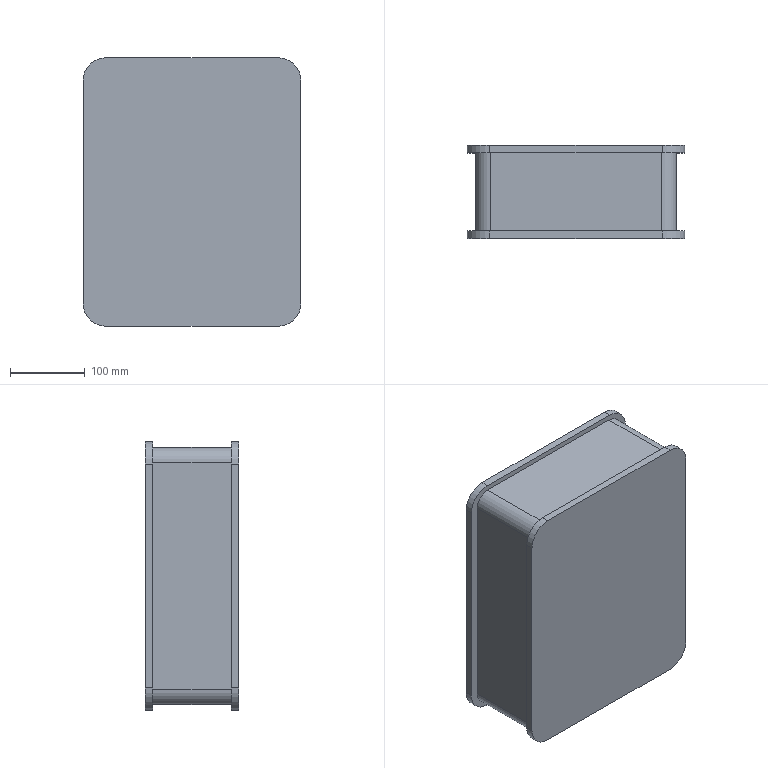Part | STEP file | CONTENEDOR TORNILLOS | 1 solid | 37 faces | box 292 x 125 x 360 mm | volume 3821373 mm3 | plane 21 | cylinder 16 | commonest cylinder face diameters 40 x8 60 x8
STEP:
#1=CARTESIAN_POINT('',(146.,125.,150.));
#2=VERTEX_POINT('',#1);
#3=CARTESIAN_POINT('',(146.,115.,150.));
#4=VERTEX_POINT('',#3);
#5=CARTESIAN_POINT('',(146.,125.,150.));
#6=DIRECTION('',(0.,-1.,0.));
#7=VECTOR('',#6,1000.);
#8=LINE('',#5,#7);
#9=EDGE_CURVE('',#2,#4,#8,.T.);
#10=ORIENTED_EDGE('',*,*,#9,.T.);
#11=CARTESIAN_POINT('',(146.,115.,-150.));
#12=VERTEX_POINT('',#11);
#13=CARTESIAN_POINT('',(146.,115.,180.));
#14=DIRECTION('',(0.,0.,-1.));
#15=VECTOR('',#14,1000.);
#16=LINE('',#13,#15);
#17=EDGE_CURVE('',#4,#12,#16,.T.);
#18=ORIENTED_EDGE('',*,*,#17,.T.);
#19=CARTESIAN_POINT('',(146.,125.,-150.));
#20=VERTEX_POINT('',#19);
#21=CARTESIAN_POINT('',(146.,125.,-150.));
#22=DIRECTION('',(0.,1.,0.));
#23=VECTOR('',#22,1000.);
#24=LINE('',#21,#23);
#25=EDGE_CURVE('',#12,#20,#24,.T.);
#26=ORIENTED_EDGE('',*,*,#25,.T.);
#27=CARTESIAN_POINT('',(146.,125.,180.));
#28=DIRECTION('',(0.,0.,-1.));
#29=VECTOR('',#28,1000.);
#30=LINE('',#27,#29);
#31=EDGE_CURVE('',#2,#20,#30,.T.);
#32=ORIENTED_EDGE('',*,*,#31,.F.);
#33=EDGE_LOOP('',(#10,#18,#26,#32));
#34=FACE_OUTER_BOUND('',#33,.T.);
#35=CARTESIAN_POINT('',(146.,125.,180.));
#36=DIRECTION('',(-1.,0.,0.));
#37=DIRECTION('',(0.,0.,1.));
#38=AXIS2_PLACEMENT_3D('',#35,#36,#37);
#39=PLANE('',#38);
#40=ADVANCED_FACE('',(#34),#39,.F.);
#41=CARTESIAN_POINT('',(116.,125.,-180.));
#42=VERTEX_POINT('',#41);
#43=CARTESIAN_POINT('',(116.,115.,-180.));
#44=VERTEX_POINT('',#43);
#45=CARTESIAN_POINT('',(116.,125.,-180.));
#46=DIRECTION('',(0.,-1.,0.));
#47=VECTOR('',#46,1000.);
#48=LINE('',#45,#47);
#49=EDGE_CURVE('',#42,#44,#48,.T.);
#50=ORIENTED_EDGE('',*,*,#49,.T.);
#51=CARTESIAN_POINT('',(-116.,115.,-180.));
#52=VERTEX_POINT('',#51);
#53=CARTESIAN_POINT('',(-146.,115.,-180.));
#54=DIRECTION('',(-1.,0.,0.));
#55=VECTOR('',#54,1000.);
#56=LINE('',#53,#55);
#57=EDGE_CURVE('',#44,#52,#56,.T.);
#58=ORIENTED_EDGE('',*,*,#57,.T.);
#59=CARTESIAN_POINT('',(-116.,125.,-180.));
#60=VERTEX_POINT('',#59);
#61=CARTESIAN_POINT('',(-116.,125.,-180.));
#62=DIRECTION('',(0.,1.,0.));
#63=VECTOR('',#62,1000.);
#64=LINE('',#61,#63);
#65=EDGE_CURVE('',#52,#60,#64,.T.);
#66=ORIENTED_EDGE('',*,*,#65,.T.);
#67=CARTESIAN_POINT('',(-146.,125.,-180.));
#68=DIRECTION('',(-1.,0.,0.));
#69=VECTOR('',#68,1000.);
#70=LINE('',#67,#69);
#71=EDGE_CURVE('',#42,#60,#70,.T.);
#72=ORIENTED_EDGE('',*,*,#71,.F.);
#73=EDGE_LOOP('',(#50,#58,#66,#72));
#74=FACE_OUTER_BOUND('',#73,.T.);
#75=CARTESIAN_POINT('',(-146.,125.,-180.));
#76=DIRECTION('',(0.,0.,1.));
#77=DIRECTION('',(1.,0.,0.));
#78=AXIS2_PLACEMENT_3D('',#75,#76,#77);
#79=PLANE('',#78);
#80=ADVANCED_FACE('',(#74),#79,.F.);
#81=CARTESIAN_POINT('',(-146.,125.,-150.));
#82=VERTEX_POINT('',#81);
#83=CARTESIAN_POINT('',(-146.,115.,-150.));
#84=VERTEX_POINT('',#83);
#85=CARTESIAN_POINT('',(-146.,125.,-150.));
#86=DIRECTION('',(0.,-1.,0.));
#87=VECTOR('',#86,1000.);
#88=LINE('',#85,#87);
#89=EDGE_CURVE('',#82,#84,#88,.T.);
#90=ORIENTED_EDGE('',*,*,#89,.T.);
#91=CARTESIAN_POINT('',(-146.,115.,150.));
#92=VERTEX_POINT('',#91);
#93=CARTESIAN_POINT('',(-146.,115.,180.));
#94=DIRECTION('',(0.,0.,1.));
#95=VECTOR('',#94,1000.);
#96=LINE('',#93,#95);
#97=EDGE_CURVE('',#84,#92,#96,.T.);
#98=ORIENTED_EDGE('',*,*,#97,.T.);
#99=CARTESIAN_POINT('',(-146.,125.,150.));
#100=VERTEX_POINT('',#99);
#101=CARTESIAN_POINT('',(-146.,125.,150.));
#102=DIRECTION('',(0.,1.,0.));
#103=VECTOR('',#102,1000.);
#104=LINE('',#101,#103);
#105=EDGE_CURVE('',#92,#100,#104,.T.);
#106=ORIENTED_EDGE('',*,*,#105,.T.);
#107=CARTESIAN_POINT('',(-146.,125.,180.));
#108=DIRECTION('',(0.,0.,1.));
#109=VECTOR('',#108,1000.);
#110=LINE('',#107,#109);
#111=EDGE_CURVE('',#82,#100,#110,.T.);
#112=ORIENTED_EDGE('',*,*,#111,.F.);
#113=EDGE_LOOP('',(#90,#98,#106,#112));
#114=FACE_OUTER_BOUND('',#113,.T.);
#115=CARTESIAN_POINT('',(-146.,125.,180.));
#116=DIRECTION('',(1.,0.,0.));
#117=DIRECTION('',(0.,0.,-1.));
#118=AXIS2_PLACEMENT_3D('',#115,#116,#117);
#119=PLANE('',#118);
#120=ADVANCED_FACE('',(#114),#119,.F.);
#121=CARTESIAN_POINT('',(-116.,125.,180.));
#122=VERTEX_POINT('',#121);
#123=CARTESIAN_POINT('',(-116.,115.,180.));
#124=VERTEX_POINT('',#123);
#125=CARTESIAN_POINT('',(-116.,125.,180.));
#126=DIRECTION('',(0.,-1.,0.));
#127=VECTOR('',#126,1000.);
#128=LINE('',#125,#127);
#129=EDGE_CURVE('',#122,#124,#128,.T.);
#130=ORIENTED_EDGE('',*,*,#129,.T.);
#131=CARTESIAN_POINT('',(116.,115.,180.));
#132=VERTEX_POINT('',#131);
#133=CARTESIAN_POINT('',(-146.,115.,180.));
#134=DIRECTION('',(1.,0.,0.));
#135=VECTOR('',#134,1000.);
#136=LINE('',#133,#135);
#137=EDGE_CURVE('',#124,#132,#136,.T.);
#138=ORIENTED_EDGE('',*,*,#137,.T.);
#139=CARTESIAN_POINT('',(116.,125.,180.));
#140=VERTEX_POINT('',#139);
#141=CARTESIAN_POINT('',(116.,125.,180.));
#142=DIRECTION('',(0.,1.,0.));
#143=VECTOR('',#142,1000.);
#144=LINE('',#141,#143);
#145=EDGE_CURVE('',#132,#140,#144,.T.);
#146=ORIENTED_EDGE('',*,*,#145,.T.);
#147=CARTESIAN_POINT('',(-146.,125.,180.));
#148=DIRECTION('',(1.,0.,0.));
#149=VECTOR('',#148,1000.);
#150=LINE('',#147,#149);
#151=EDGE_CURVE('',#122,#140,#150,.T.);
#152=ORIENTED_EDGE('',*,*,#151,.F.);
#153=EDGE_LOOP('',(#130,#138,#146,#152));
#154=FACE_OUTER_BOUND('',#153,.T.);
#155=CARTESIAN_POINT('',(-146.,125.,180.));
#156=DIRECTION('',(0.,0.,-1.));
#157=DIRECTION('',(-1.,0.,0.));
#158=AXIS2_PLACEMENT_3D('',#155,#156,#157);
#159=PLANE('',#158);
#160=ADVANCED_FACE('',(#154),#159,.F.);
#161=CARTESIAN_POINT('',(125.,125.,145.));
#162=VERTEX_POINT('',#161);
#163=CARTESIAN_POINT('',(125.,125.,-145.));
#164=VERTEX_POINT('',#163);
#165=CARTESIAN_POINT('',(125.,125.,145.));
#166=DIRECTION('',(0.,0.,-1.));
#167=VECTOR('',#166,1000.);
#168=LINE('',#165,#167);
#169=EDGE_CURVE('',#162,#164,#168,.T.);
#170=ORIENTED_EDGE('',*,*,#169,.F.);
#171=CARTESIAN_POINT('',(105.,125.,165.));
#172=VERTEX_POINT('',#171);
#173=CARTESIAN_POINT('',(105.,125.,145.));
#174=DIRECTION('',(0.,1.,0.));
#175=DIRECTION('',(0.,0.,1.));
#176=AXIS2_PLACEMENT_3D('',#173,#174,#175);
#177=CIRCLE('',#176,20.);
#178=EDGE_CURVE('',#172,#162,#177,.T.);
#179=ORIENTED_EDGE('',*,*,#178,.F.);
#180=CARTESIAN_POINT('',(-105.,125.,165.));
#181=VERTEX_POINT('',#180);
#182=CARTESIAN_POINT('',(105.,125.,165.));
#183=DIRECTION('',(1.,0.,0.));
#184=VECTOR('',#183,1000.);
#185=LINE('',#182,#184);
#186=EDGE_CURVE('',#181,#172,#185,.T.);
#187=ORIENTED_EDGE('',*,*,#186,.F.);
#188=CARTESIAN_POINT('',(-125.,125.,145.));
#189=VERTEX_POINT('',#188);
#190=CARTESIAN_POINT('',(-105.,125.,145.));
#191=DIRECTION('',(0.,1.,0.));
#192=DIRECTION('',(0.,0.,-1.));
#193=AXIS2_PLACEMENT_3D('',#190,#191,#192);
#194=CIRCLE('',#193,20.);
#195=EDGE_CURVE('',#189,#181,#194,.T.);
#196=ORIENTED_EDGE('',*,*,#195,.F.);
#197=CARTESIAN_POINT('',(-125.,125.,-145.));
#198=VERTEX_POINT('',#197);
#199=CARTESIAN_POINT('',(-125.,125.,145.));
#200=DIRECTION('',(0.,0.,1.));
#201=VECTOR('',#200,1000.);
#202=LINE('',#199,#201);
#203=EDGE_CURVE('',#198,#189,#202,.T.);
#204=ORIENTED_EDGE('',*,*,#203,.F.);
#205=CARTESIAN_POINT('',(-105.,125.,-165.));
#206=VERTEX_POINT('',#205);
#207=CARTESIAN_POINT('',(-105.,125.,-145.));
#208=DIRECTION('',(0.,1.,0.));
#209=DIRECTION('',(0.,0.,1.));
#210=AXIS2_PLACEMENT_3D('',#207,#208,#209);
#211=CIRCLE('',#210,20.);
#212=EDGE_CURVE('',#206,#198,#211,.T.);
#213=ORIENTED_EDGE('',*,*,#212,.F.);
#214=CARTESIAN_POINT('',(105.,125.,-165.));
#215=VERTEX_POINT('',#214);
#216=CARTESIAN_POINT('',(105.,125.,-165.));
#217=DIRECTION('',(-1.,0.,0.));
#218=VECTOR('',#217,1000.);
#219=LINE('',#216,#218);
#220=EDGE_CURVE('',#215,#206,#219,.T.);
#221=ORIENTED_EDGE('',*,*,#220,.F.);
#222=CARTESIAN_POINT('',(105.,125.,-145.));
#223=DIRECTION('',(0.,1.,0.));
#224=DIRECTION('',(0.,0.,1.));
#225=AXIS2_PLACEMENT_3D('',#222,#223,#224);
#226=CIRCLE('',#225,20.);
#227=EDGE_CURVE('',#164,#215,#226,.T.);
#228=ORIENTED_EDGE('',*,*,#227,.F.);
#229=EDGE_LOOP('',(#170,#179,#187,#196,#204,#213,#221,#228));
#230=FACE_BOUND('',#229,.T.);
#231=ORIENTED_EDGE('',*,*,#31,.T.);
#232=CARTESIAN_POINT('',(116.,125.,-150.));
#233=DIRECTION('',(0.,1.,0.));
#234=DIRECTION('',(0.,0.,-1.));
#235=AXIS2_PLACEMENT_3D('',#232,#233,#234);
#236=CIRCLE('',#235,30.);
#237=EDGE_CURVE('',#20,#42,#236,.T.);
#238=ORIENTED_EDGE('',*,*,#237,.T.);
#239=ORIENTED_EDGE('',*,*,#71,.T.);
#240=CARTESIAN_POINT('',(-116.,125.,-150.));
#241=DIRECTION('',(0.,1.,0.));
#242=DIRECTION('',(0.,0.,-1.));
#243=AXIS2_PLACEMENT_3D('',#240,#241,#242);
#244=CIRCLE('',#243,30.);
#245=EDGE_CURVE('',#60,#82,#244,.T.);
#246=ORIENTED_EDGE('',*,*,#245,.T.);
#247=ORIENTED_EDGE('',*,*,#111,.T.);
#248=CARTESIAN_POINT('',(-116.,125.,150.));
#249=DIRECTION('',(0.,1.,0.));
#250=DIRECTION('',(0.,0.,-1.));
#251=AXIS2_PLACEMENT_3D('',#248,#249,#250);
#252=CIRCLE('',#251,30.);
#253=EDGE_CURVE('',#100,#122,#252,.T.);
#254=ORIENTED_EDGE('',*,*,#253,.T.);
#255=ORIENTED_EDGE('',*,*,#151,.T.);
#256=CARTESIAN_POINT('',(116.,125.,150.));
#257=DIRECTION('',(0.,1.,0.));
#258=DIRECTION('',(0.,0.,-1.));
#259=AXIS2_PLACEMENT_3D('',#256,#257,#258);
#260=CIRCLE('',#259,30.);
#261=EDGE_CURVE('',#140,#2,#260,.T.);
#262=ORIENTED_EDGE('',*,*,#261,.T.);
#263=EDGE_LOOP('',(#231,#238,#239,#246,#247,#254,#255,#262));
#264=FACE_OUTER_BOUND('',#263,.T.);
#265=CARTESIAN_POINT('',(0.,125.,0.));
#266=DIRECTION('',(0.,-1.,0.));
#267=DIRECTION('',(0.,0.,-1.));
#268=AXIS2_PLACEMENT_3D('',#265,#266,#267);
#269=PLANE('',#268);
#270=ADVANCED_FACE('',(#230,#264),#269,.F.);
#271=CARTESIAN_POINT('',(116.,115.,-150.));
#272=DIRECTION('',(0.,-1.,0.));
#273=DIRECTION('',(0.,0.,1.));
#274=AXIS2_PLACEMENT_3D('',#271,#272,#273);
#275=CIRCLE('',#274,30.);
#276=EDGE_CURVE('',#44,#12,#275,.T.);
#277=ORIENTED_EDGE('',*,*,#276,.F.);
#278=ORIENTED_EDGE('',*,*,#49,.F.);
#279=ORIENTED_EDGE('',*,*,#237,.F.);
#280=ORIENTED_EDGE('',*,*,#25,.F.);
#281=EDGE_LOOP('',(#277,#278,#279,#280));
#282=FACE_OUTER_BOUND('',#281,.T.);
#283=CARTESIAN_POINT('',(116.,125.,-150.));
#284=DIRECTION('',(0.,-1.,0.));
#285=DIRECTION('',(0.,0.,-1.));
#286=AXIS2_PLACEMENT_3D('',#283,#284,#285);
#287=CYLINDRICAL_SURFACE('',#286,30.);
#288=ADVANCED_FACE('',(#282),#287,.T.);
#289=CARTESIAN_POINT('',(-116.,115.,-150.));
#290=DIRECTION('',(0.,-1.,0.));
#291=DIRECTION('',(0.,0.,1.));
#292=AXIS2_PLACEMENT_3D('',#289,#290,#291);
#293=CIRCLE('',#292,30.);
#294=EDGE_CURVE('',#84,#52,#293,.T.);
#295=ORIENTED_EDGE('',*,*,#294,.F.);
#296=ORIENTED_EDGE('',*,*,#89,.F.);
#297=ORIENTED_EDGE('',*,*,#245,.F.);
#298=ORIENTED_EDGE('',*,*,#65,.F.);
#299=EDGE_LOOP('',(#295,#296,#297,#298));
#300=FACE_OUTER_BOUND('',#299,.T.);
#301=CARTESIAN_POINT('',(-116.,125.,-150.));
#302=DIRECTION('',(0.,-1.,0.));
#303=DIRECTION('',(0.,0.,-1.));
#304=AXIS2_PLACEMENT_3D('',#301,#302,#303);
#305=CYLINDRICAL_SURFACE('',#304,30.);
#306=ADVANCED_FACE('',(#300),#305,.T.);
#307=CARTESIAN_POINT('',(116.,115.,150.));
#308=DIRECTION('',(0.,-1.,0.));
#309=DIRECTION('',(0.,0.,1.));
#310=AXIS2_PLACEMENT_3D('',#307,#308,#309);
#311=CIRCLE('',#310,30.);
#312=EDGE_CURVE('',#4,#132,#311,.T.);
#313=ORIENTED_EDGE('',*,*,#312,.F.);
#314=ORIENTED_EDGE('',*,*,#9,.F.);
#315=ORIENTED_EDGE('',*,*,#261,.F.);
#316=ORIENTED_EDGE('',*,*,#145,.F.);
#317=EDGE_LOOP('',(#313,#314,#315,#316));
#318=FACE_OUTER_BOUND('',#317,.T.);
#319=CARTESIAN_POINT('',(116.,125.,150.));
#320=DIRECTION('',(0.,-1.,0.));
#321=DIRECTION('',(0.,0.,-1.));
#322=AXIS2_PLACEMENT_3D('',#319,#320,#321);
#323=CYLINDRICAL_SURFACE('',#322,30.);
#324=ADVANCED_FACE('',(#318),#323,.T.);
#325=CARTESIAN_POINT('',(-116.,115.,150.));
#326=DIRECTION('',(0.,-1.,0.));
#327=DIRECTION('',(0.,0.,1.));
#328=AXIS2_PLACEMENT_3D('',#325,#326,#327);
#329=CIRCLE('',#328,30.);
#330=EDGE_CURVE('',#124,#92,#329,.T.);
#331=ORIENTED_EDGE('',*,*,#330,.F.);
#332=ORIENTED_EDGE('',*,*,#129,.F.);
#333=ORIENTED_EDGE('',*,*,#253,.F.);
#334=ORIENTED_EDGE('',*,*,#105,.F.);
#335=EDGE_LOOP('',(#331,#332,#333,#334));
#336=FACE_OUTER_BOUND('',#335,.T.);
#337=CARTESIAN_POINT('',(-116.,125.,150.));
#338=DIRECTION('',(0.,-1.,0.));
#339=DIRECTION('',(0.,0.,-1.));
#340=AXIS2_PLACEMENT_3D('',#337,#338,#339);
#341=CYLINDRICAL_SURFACE('',#340,30.);
#342=ADVANCED_FACE('',(#336),#341,.T.);
#343=ORIENTED_EDGE('',*,*,#178,.T.);
#344=CARTESIAN_POINT('',(125.,27.5,145.));
#345=VERTEX_POINT('',#344);
#346=CARTESIAN_POINT('',(125.,27.5,145.));
#347=DIRECTION('',(0.,1.,0.));
#348=VECTOR('',#347,1000.);
#349=LINE('',#346,#348);
#350=EDGE_CURVE('',#345,#162,#349,.T.);
#351=ORIENTED_EDGE('',*,*,#350,.F.);
#352=CARTESIAN_POINT('',(105.,27.5,165.));
#353=VERTEX_POINT('',#352);
#354=CARTESIAN_POINT('',(105.,27.5,145.));
#355=DIRECTION('',(0.,1.,0.));
#356=DIRECTION('',(0.,0.,1.));
#357=AXIS2_PLACEMENT_3D('',#354,#355,#356);
#358=CIRCLE('',#357,20.);
#359=EDGE_CURVE('',#353,#345,#358,.T.);
#360=ORIENTED_EDGE('',*,*,#359,.F.);
#361=CARTESIAN_POINT('',(105.,27.5,165.));
#362=DIRECTION('',(0.,1.,0.));
#363=VECTOR('',#362,1000.);
#364=LINE('',#361,#363);
#365=EDGE_CURVE('',#353,#172,#364,.T.);
#366=ORIENTED_EDGE('',*,*,#365,.T.);
#367=EDGE_LOOP('',(#343,#351,#360,#366));
#368=FACE_OUTER_BOUND('',#367,.T.);
#369=CARTESIAN_POINT('',(105.,27.5,145.));
#370=DIRECTION('',(0.,1.,0.));
#371=DIRECTION('',(0.,0.,1.));
#372=AXIS2_PLACEMENT_3D('',#369,#370,#371);
#373=CYLINDRICAL_SURFACE('',#372,20.);
#374=ADVANCED_FACE('',(#368),#373,.F.);
#375=ORIENTED_EDGE('',*,*,#186,.T.);
#376=ORIENTED_EDGE('',*,*,#365,.F.);
#377=CARTESIAN_POINT('',(-105.,27.5,165.));
#378=VERTEX_POINT('',#377);
#379=CARTESIAN_POINT('',(105.,27.5,165.));
#380=DIRECTION('',(1.,0.,0.));
#381=VECTOR('',#380,1000.);
#382=LINE('',#379,#381);
#383=EDGE_CURVE('',#378,#353,#382,.T.);
#384=ORIENTED_EDGE('',*,*,#383,.F.);
#385=CARTESIAN_POINT('',(-105.,27.5,165.));
#386=DIRECTION('',(0.,1.,0.));
#387=VECTOR('',#386,1000.);
#388=LINE('',#385,#387);
#389=EDGE_CURVE('',#378,#181,#388,.T.);
#390=ORIENTED_EDGE('',*,*,#389,.T.);
#391=EDGE_LOOP('',(#375,#376,#384,#390));
#392=FACE_OUTER_BOUND('',#391,.T.);
#393=CARTESIAN_POINT('',(105.,27.5,165.));
#394=DIRECTION('',(0.,0.,1.));
#395=DIRECTION('',(1.,0.,0.));
#396=AXIS2_PLACEMENT_3D('',#393,#394,#395);
#397=PLANE('',#396);
#398=ADVANCED_FACE('',(#392),#397,.F.);
#399=ORIENTED_EDGE('',*,*,#195,.T.);
#400=ORIENTED_EDGE('',*,*,#389,.F.);
#401=CARTESIAN_POINT('',(-125.,27.5,145.));
#402=VERTEX_POINT('',#401);
#403=CARTESIAN_POINT('',(-105.,27.5,145.));
#404=DIRECTION('',(0.,1.,0.));
#405=DIRECTION('',(0.,0.,-1.));
#406=AXIS2_PLACEMENT_3D('',#403,#404,#405);
#407=CIRCLE('',#406,20.);
#408=EDGE_CURVE('',#402,#378,#407,.T.);
#409=ORIENTED_EDGE('',*,*,#408,.F.);
#410=CARTESIAN_POINT('',(-125.,27.5,145.));
#411=DIRECTION('',(0.,1.,0.));
#412=VECTOR('',#411,1000.);
#413=LINE('',#410,#412);
#414=EDGE_CURVE('',#402,#189,#413,.T.);
#415=ORIENTED_EDGE('',*,*,#414,.T.);
#416=EDGE_LOOP('',(#399,#400,#409,#415));
#417=FACE_OUTER_BOUND('',#416,.T.);
#418=CARTESIAN_POINT('',(-105.,27.5,145.));
#419=DIRECTION('',(0.,1.,0.));
#420=DIRECTION('',(0.,0.,1.));
#421=AXIS2_PLACEMENT_3D('',#418,#419,#420);
#422=CYLINDRICAL_SURFACE('',#421,20.);
#423=ADVANCED_FACE('',(#417),#422,.F.);
#424=ORIENTED_EDGE('',*,*,#203,.T.);
#425=ORIENTED_EDGE('',*,*,#414,.F.);
#426=CARTESIAN_POINT('',(-125.,27.5,-145.));
#427=VERTEX_POINT('',#426);
#428=CARTESIAN_POINT('',(-125.,27.5,145.));
#429=DIRECTION('',(0.,0.,1.));
#430=VECTOR('',#429,1000.);
#431=LINE('',#428,#430);
#432=EDGE_CURVE('',#427,#402,#431,.T.);
#433=ORIENTED_EDGE('',*,*,#432,.F.);
#434=CARTESIAN_POINT('',(-125.,27.5,-145.));
#435=DIRECTION('',(0.,1.,0.));
#436=VECTOR('',#435,1000.);
#437=LINE('',#434,#436);
#438=EDGE_CURVE('',#427,#198,#437,.T.);
#439=ORIENTED_EDGE('',*,*,#438,.T.);
#440=EDGE_LOOP('',(#424,#425,#433,#439));
#441=FACE_OUTER_BOUND('',#440,.T.);
#442=CARTESIAN_POINT('',(-125.,27.5,145.));
#443=DIRECTION('',(-1.,0.,0.));
#444=DIRECTION('',(0.,0.,1.));
#445=AXIS2_PLACEMENT_3D('',#442,#443,#444);
#446=PLANE('',#445);
#447=ADVANCED_FACE('',(#441),#446,.F.);
#448=ORIENTED_EDGE('',*,*,#212,.T.);
#449=ORIENTED_EDGE('',*,*,#438,.F.);
#450=CARTESIAN_POINT('',(-105.,27.5,-165.));
#451=VERTEX_POINT('',#450);
#452=CARTESIAN_POINT('',(-105.,27.5,-145.));
#453=DIRECTION('',(0.,1.,0.));
#454=DIRECTION('',(0.,0.,1.));
#455=AXIS2_PLACEMENT_3D('',#452,#453,#454);
#456=CIRCLE('',#455,20.);
#457=EDGE_CURVE('',#451,#427,#456,.T.);
#458=ORIENTED_EDGE('',*,*,#457,.F.);
#459=CARTESIAN_POINT('',(-105.,27.5,-165.));
#460=DIRECTION('',(0.,1.,0.));
#461=VECTOR('',#460,1000.);
#462=LINE('',#459,#461);
#463=EDGE_CURVE('',#451,#206,#462,.T.);
#464=ORIENTED_EDGE('',*,*,#463,.T.);
#465=EDGE_LOOP('',(#448,#449,#458,#464));
#466=FACE_OUTER_BOUND('',#465,.T.);
#467=CARTESIAN_POINT('',(-105.,27.5,-145.));
#468=DIRECTION('',(0.,1.,0.));
#469=DIRECTION('',(0.,0.,1.));
#470=AXIS2_PLACEMENT_3D('',#467,#468,#469);
#471=CYLINDRICAL_SURFACE('',#470,20.);
#472=ADVANCED_FACE('',(#466),#471,.F.);
#473=ORIENTED_EDGE('',*,*,#220,.T.);
#474=ORIENTED_EDGE('',*,*,#463,.F.);
#475=CARTESIAN_POINT('',(105.,27.5,-165.));
#476=VERTEX_POINT('',#475);
#477=CARTESIAN_POINT('',(105.,27.5,-165.));
#478=DIRECTION('',(-1.,0.,0.));
#479=VECTOR('',#478,1000.);
#480=LINE('',#477,#479);
#481=EDGE_CURVE('',#476,#451,#480,.T.);
#482=ORIENTED_EDGE('',*,*,#481,.F.);
#483=CARTESIAN_POINT('',(105.,27.5,-165.));
#484=DIRECTION('',(0.,1.,0.));
#485=VECTOR('',#484,1000.);
#486=LINE('',#483,#485);
#487=EDGE_CURVE('',#476,#215,#486,.T.);
#488=ORIENTED_EDGE('',*,*,#487,.T.);
#489=EDGE_LOOP('',(#473,#474,#482,#488));
#490=FACE_OUTER_BOUND('',#489,.T.);
#491=CARTESIAN_POINT('',(105.,27.5,-165.));
#492=DIRECTION('',(0.,0.,-1.));
#493=DIRECTION('',(-1.,0.,0.));
#494=AXIS2_PLACEMENT_3D('',#491,#492,#493);
#495=PLANE('',#494);
#496=ADVANCED_FACE('',(#490),#495,.F.);
#497=ORIENTED_EDGE('',*,*,#227,.T.);
#498=ORIENTED_EDGE('',*,*,#487,.F.);
#499=CARTESIAN_POINT('',(125.,27.5,-145.));
#500=VERTEX_POINT('',#499);
#501=CARTESIAN_POINT('',(105.,27.5,-145.));
#502=DIRECTION('',(0.,1.,0.));
#503=DIRECTION('',(0.,0.,1.));
#504=AXIS2_PLACEMENT_3D('',#501,#502,#503);
#505=CIRCLE('',#504,20.);
#506=EDGE_CURVE('',#500,#476,#505,.T.);
#507=ORIENTED_EDGE('',*,*,#506,.F.);
#508=CARTESIAN_POINT('',(125.,27.5,-145.));
#509=DIRECTION('',(0.,1.,0.));
#510=VECTOR('',#509,1000.);
#511=LINE('',#508,#510);
#512=EDGE_CURVE('',#500,#164,#511,.T.);
#513=ORIENTED_EDGE('',*,*,#512,.T.);
#514=EDGE_LOOP('',(#497,#498,#507,#513));
#515=FACE_OUTER_BOUND('',#514,.T.);
#516=CARTESIAN_POINT('',(105.,27.5,-145.));
#517=DIRECTION('',(0.,1.,0.));
#518=DIRECTION('',(0.,0.,1.));
#519=AXIS2_PLACEMENT_3D('',#516,#517,#518);
#520=CYLINDRICAL_SURFACE('',#519,20.);
#521=ADVANCED_FACE('',(#515),#520,.F.);
#522=ORIENTED_EDGE('',*,*,#169,.T.);
#523=ORIENTED_EDGE('',*,*,#512,.F.);
#524=CARTESIAN_POINT('',(125.,27.5,145.));
#525=DIRECTION('',(0.,0.,-1.));
#526=VECTOR('',#525,1000.);
#527=LINE('',#524,#526);
#528=EDGE_CURVE('',#345,#500,#527,.T.);
#529=ORIENTED_EDGE('',*,*,#528,.F.);
#530=ORIENTED_EDGE('',*,*,#350,.T.);
#531=EDGE_LOOP('',(#522,#523,#529,#530));
#532=FACE_OUTER_BOUND('',#531,.T.);
#533=CARTESIAN_POINT('',(125.,27.5,145.));
#534=DIRECTION('',(1.,0.,0.));
#535=DIRECTION('',(0.,0.,-1.));
#536=AXIS2_PLACEMENT_3D('',#533,#534,#535);
#537=PLANE('',#536);
#538=ADVANCED_FACE('',(#532),#537,.F.);
#539=ORIENTED_EDGE('',*,*,#359,.T.);
#540=ORIENTED_EDGE('',*,*,#528,.T.);
#541=ORIENTED_EDGE('',*,*,#506,.T.);
#542=ORIENTED_EDGE('',*,*,#481,.T.);
#543=ORIENTED_EDGE('',*,*,#457,.T.);
#544=ORIENTED_EDGE('',*,*,#432,.T.);
#545=ORIENTED_EDGE('',*,*,#408,.T.);
#546=ORIENTED_EDGE('',*,*,#383,.T.);
#547=EDGE_LOOP('',(#539,#540,#541,#542,#543,#544,#545,#546));
#548=FACE_OUTER_BOUND('',#547,.T.);
#549=CARTESIAN_POINT('',(105.,27.5,145.));
#550=DIRECTION('',(0.,1.,0.));
#551=DIRECTION('',(0.,0.,1.));
#552=AXIS2_PLACEMENT_3D('',#549,#550,#551);
#553=PLANE('',#552);
#554=ADVANCED_FACE('',(#548),#553,.T.);
#555=CARTESIAN_POINT('',(-115.,115.,172.5));
#556=VERTEX_POINT('',#555);
#557=CARTESIAN_POINT('',(-135.,115.,152.5));
#558=VERTEX_POINT('',#557);
#559=CARTESIAN_POINT('',(-115.,115.,152.5));
#560=DIRECTION('',(0.,-1.,0.));
#561=DIRECTION('',(0.,0.,1.));
#562=AXIS2_PLACEMENT_3D('',#559,#560,#561);
#563=CIRCLE('',#562,20.);
#564=EDGE_CURVE('',#556,#558,#563,.T.);
#565=ORIENTED_EDGE('',*,*,#564,.T.);
#566=CARTESIAN_POINT('',(-135.,10.,152.5));
#567=VERTEX_POINT('',#566);
#568=CARTESIAN_POINT('',(-135.,583.17,152.5));
#569=DIRECTION('',(0.,-1.,0.));
#570=VECTOR('',#569,1000.);
#571=LINE('',#568,#570);
#572=EDGE_CURVE('',#558,#567,#571,.T.);
#573=ORIENTED_EDGE('',*,*,#572,.T.);
#574=CARTESIAN_POINT('',(-115.,10.,172.5));
#575=VERTEX_POINT('',#574);
#576=CARTESIAN_POINT('',(-115.,10.,152.5));
#577=DIRECTION('',(0.,-1.,0.));
#578=DIRECTION('',(0.,0.,-1.));
#579=AXIS2_PLACEMENT_3D('',#576,#577,#578);
#580=CIRCLE('',#579,20.);
#581=EDGE_CURVE('',#575,#567,#580,.T.);
#582=ORIENTED_EDGE('',*,*,#581,.F.);
#583=CARTESIAN_POINT('',(-115.,583.17,172.5));
#584=DIRECTION('',(0.,-1.,0.));
#585=VECTOR('',#584,1000.);
#586=LINE('',#583,#585);
#587=EDGE_CURVE('',#556,#575,#586,.T.);
#588=ORIENTED_EDGE('',*,*,#587,.F.);
#589=EDGE_LOOP('',(#565,#573,#582,#588));
#590=FACE_OUTER_BOUND('',#589,.T.);
#591=CARTESIAN_POINT('',(-115.,583.17,152.5));
#592=DIRECTION('',(0.,-1.,0.));
#593=DIRECTION('',(0.,0.,-1.));
#594=AXIS2_PLACEMENT_3D('',#591,#592,#593);
#595=CYLINDRICAL_SURFACE('',#594,20.);
#596=ADVANCED_FACE('',(#590),#595,.T.);
#597=ORIENTED_EDGE('',*,*,#587,.T.);
#598=CARTESIAN_POINT('',(115.,10.,172.5));
#599=VERTEX_POINT('',#598);
#600=CARTESIAN_POINT('',(-115.,10.,172.5));
#601=DIRECTION('',(1.,0.,0.));
#602=VECTOR('',#601,1000.);
#603=LINE('',#600,#602);
#604=EDGE_CURVE('',#575,#599,#603,.T.);
#605=ORIENTED_EDGE('',*,*,#604,.T.);
#606=CARTESIAN_POINT('',(115.,115.,172.5));
#607=VERTEX_POINT('',#606);
#608=CARTESIAN_POINT('',(115.,583.17,172.5));
#609=DIRECTION('',(0.,-1.,0.));
#610=VECTOR('',#609,1000.);
#611=LINE('',#608,#610);
#612=EDGE_CURVE('',#607,#599,#611,.T.);
#613=ORIENTED_EDGE('',*,*,#612,.F.);
#614=CARTESIAN_POINT('',(-115.,115.,172.5));
#615=DIRECTION('',(1.,0.,0.));
#616=VECTOR('',#615,1000.);
#617=LINE('',#614,#616);
#618=EDGE_CURVE('',#556,#607,#617,.T.);
#619=ORIENTED_EDGE('',*,*,#618,.F.);
#620=EDGE_LOOP('',(#597,#605,#613,#619));
#621=FACE_OUTER_BOUND('',#620,.T.);
#622=CARTESIAN_POINT('',(-115.,583.17,172.5));
#623=DIRECTION('',(0.,0.,-1.));
#624=DIRECTION('',(-1.,0.,0.));
#625=AXIS2_PLACEMENT_3D('',#622,#623,#624);
#626=PLANE('',#625);
#627=ADVANCED_FACE('',(#621),#626,.F.);
#628=ORIENTED_EDGE('',*,*,#612,.T.);
#629=CARTESIAN_POINT('',(135.,10.,152.5));
#630=VERTEX_POINT('',#629);
#631=CARTESIAN_POINT('',(115.,10.,152.5));
#632=DIRECTION('',(0.,1.,0.));
#633=DIRECTION('',(0.,0.,1.));
#634=AXIS2_PLACEMENT_3D('',#631,#632,#633);
#635=CIRCLE('',#634,20.);
#636=EDGE_CURVE('',#599,#630,#635,.T.);
#637=ORIENTED_EDGE('',*,*,#636,.T.);
#638=CARTESIAN_POINT('',(135.,115.,152.5));
#639=VERTEX_POINT('',#638);
#640=CARTESIAN_POINT('',(135.,583.17,152.5));
#641=DIRECTION('',(0.,-1.,0.));
#642=VECTOR('',#641,1000.);
#643=LINE('',#640,#642);
#644=EDGE_CURVE('',#639,#630,#643,.T.);
#645=ORIENTED_EDGE('',*,*,#644,.F.);
#646=CARTESIAN_POINT('',(115.,115.,152.5));
#647=DIRECTION('',(0.,1.,0.));
#648=DIRECTION('',(0.,0.,1.));
#649=AXIS2_PLACEMENT_3D('',#646,#647,#648);
#650=CIRCLE('',#649,20.);
#651=EDGE_CURVE('',#607,#639,#650,.T.);
#652=ORIENTED_EDGE('',*,*,#651,.F.);
#653=EDGE_LOOP('',(#628,#637,#645,#652));
#654=FACE_OUTER_BOUND('',#653,.T.);
#655=CARTESIAN_POINT('',(115.,583.17,152.5));
#656=DIRECTION('',(0.,-1.,0.));
#657=DIRECTION('',(0.,0.,-1.));
#658=AXIS2_PLACEMENT_3D('',#655,#656,#657);
#659=CYLINDRICAL_SURFACE('',#658,20.);
#660=ADVANCED_FACE('',(#654),#659,.T.);
#661=ORIENTED_EDGE('',*,*,#644,.T.);
#662=CARTESIAN_POINT('',(135.,10.,-152.5));
#663=VERTEX_POINT('',#662);
#664=CARTESIAN_POINT('',(135.,10.,152.5));
#665=DIRECTION('',(0.,0.,-1.));
#666=VECTOR('',#665,1000.);
#667=LINE('',#664,#666);
#668=EDGE_CURVE('',#630,#663,#667,.T.);
#669=ORIENTED_EDGE('',*,*,#668,.T.);
#670=CARTESIAN_POINT('',(135.,115.,-152.5));
#671=VERTEX_POINT('',#670);
#672=CARTESIAN_POINT('',(135.,583.17,-152.5));
#673=DIRECTION('',(0.,-1.,0.));
#674=VECTOR('',#673,1000.);
#675=LINE('',#672,#674);
#676=EDGE_CURVE('',#671,#663,#675,.T.);
#677=ORIENTED_EDGE('',*,*,#676,.F.);
#678=CARTESIAN_POINT('',(135.,115.,152.5));
#679=DIRECTION('',(0.,0.,-1.));
#680=VECTOR('',#679,1000.);
#681=LINE('',#678,#680);
#682=EDGE_CURVE('',#639,#671,#681,.T.);
#683=ORIENTED_EDGE('',*,*,#682,.F.);
#684=EDGE_LOOP('',(#661,#669,#677,#683));
#685=FACE_OUTER_BOUND('',#684,.T.);
#686=CARTESIAN_POINT('',(135.,583.17,152.5));
#687=DIRECTION('',(-1.,0.,0.));
#688=DIRECTION('',(0.,0.,1.));
#689=AXIS2_PLACEMENT_3D('',#686,#687,#688);
#690=PLANE('',#689);
#691=ADVANCED_FACE('',(#685),#690,.F.);
#692=CARTESIAN_POINT('',(115.,115.,-172.5));
#693=VERTEX_POINT('',#692);
#694=CARTESIAN_POINT('',(115.,115.,-152.5));
#695=DIRECTION('',(0.,-1.,0.));
#696=DIRECTION('',(0.,0.,1.));
#697=AXIS2_PLACEMENT_3D('',#694,#695,#696);
#698=CIRCLE('',#697,20.);
#699=EDGE_CURVE('',#693,#671,#698,.T.);
#700=ORIENTED_EDGE('',*,*,#699,.T.);
#701=ORIENTED_EDGE('',*,*,#676,.T.);
#702=CARTESIAN_POINT('',(115.,10.,-172.5));
#703=VERTEX_POINT('',#702);
#704=CARTESIAN_POINT('',(115.,10.,-152.5));
#705=DIRECTION('',(0.,-1.,0.));
#706=DIRECTION('',(0.,0.,-1.));
#707=AXIS2_PLACEMENT_3D('',#704,#705,#706);
#708=CIRCLE('',#707,20.);
#709=EDGE_CURVE('',#703,#663,#708,.T.);
#710=ORIENTED_EDGE('',*,*,#709,.F.);
#711=CARTESIAN_POINT('',(115.,583.17,-172.5));
#712=DIRECTION('',(0.,-1.,0.));
#713=VECTOR('',#712,1000.);
#714=LINE('',#711,#713);
#715=EDGE_CURVE('',#693,#703,#714,.T.);
#716=ORIENTED_EDGE('',*,*,#715,.F.);
#717=EDGE_LOOP('',(#700,#701,#710,#716));
#718=FACE_OUTER_BOUND('',#717,.T.);
#719=CARTESIAN_POINT('',(115.,583.17,-152.5));
#720=DIRECTION('',(0.,-1.,0.));
#721=DIRECTION('',(0.,0.,-1.));
#722=AXIS2_PLACEMENT_3D('',#719,#720,#721);
#723=CYLINDRICAL_SURFACE('',#722,20.);
#724=ADVANCED_FACE('',(#718),#723,.T.);
#725=CARTESIAN_POINT('',(-115.,115.,-172.5));
#726=VERTEX_POINT('',#725);
#727=CARTESIAN_POINT('',(-115.,115.,-172.5));
#728=DIRECTION('',(1.,0.,0.));
#729=VECTOR('',#728,1000.);
#730=LINE('',#727,#729);
#731=EDGE_CURVE('',#726,#693,#730,.T.);
#732=ORIENTED_EDGE('',*,*,#731,.T.);
#733=ORIENTED_EDGE('',*,*,#715,.T.);
#734=CARTESIAN_POINT('',(-115.,10.,-172.5));
#735=VERTEX_POINT('',#734);
#736=CARTESIAN_POINT('',(-115.,10.,-172.5));
#737=DIRECTION('',(1.,0.,0.));
#738=VECTOR('',#737,1000.);
#739=LINE('',#736,#738);
#740=EDGE_CURVE('',#735,#703,#739,.T.);
#741=ORIENTED_EDGE('',*,*,#740,.F.);
#742=CARTESIAN_POINT('',(-115.,583.17,-172.5));
#743=DIRECTION('',(0.,-1.,0.));
#744=VECTOR('',#743,1000.);
#745=LINE('',#742,#744);
#746=EDGE_CURVE('',#726,#735,#745,.T.);
#747=ORIENTED_EDGE('',*,*,#746,.F.);
#748=EDGE_LOOP('',(#732,#733,#741,#747));
#749=FACE_OUTER_BOUND('',#748,.T.);
#750=CARTESIAN_POINT('',(-115.,583.17,-172.5));
#751=DIRECTION('',(0.,0.,-1.));
#752=DIRECTION('',(-1.,0.,0.));
#753=AXIS2_PLACEMENT_3D('',#750,#751,#752);
#754=PLANE('',#753);
#755=ADVANCED_FACE('',(#749),#754,.T.);
#756=CARTESIAN_POINT('',(-135.,115.,-152.5));
#757=VERTEX_POINT('',#756);
#758=CARTESIAN_POINT('',(-115.,115.,-152.5));
#759=DIRECTION('',(0.,-1.,0.));
#760=DIRECTION('',(0.,0.,1.));
#761=AXIS2_PLACEMENT_3D('',#758,#759,#760);
#762=CIRCLE('',#761,20.);
#763=EDGE_CURVE('',#757,#726,#762,.T.);
#764=ORIENTED_EDGE('',*,*,#763,.T.);
#765=ORIENTED_EDGE('',*,*,#746,.T.);
#766=CARTESIAN_POINT('',(-135.,10.,-152.5));
#767=VERTEX_POINT('',#766);
#768=CARTESIAN_POINT('',(-115.,10.,-152.5));
#769=DIRECTION('',(0.,-1.,0.));
#770=DIRECTION('',(0.,0.,-1.));
#771=AXIS2_PLACEMENT_3D('',#768,#769,#770);
#772=CIRCLE('',#771,20.);
#773=EDGE_CURVE('',#767,#735,#772,.T.);
#774=ORIENTED_EDGE('',*,*,#773,.F.);
#775=CARTESIAN_POINT('',(-135.,583.17,-152.5));
#776=DIRECTION('',(0.,-1.,0.));
#777=VECTOR('',#776,1000.);
#778=LINE('',#775,#777);
#779=EDGE_CURVE('',#757,#767,#778,.T.);
#780=ORIENTED_EDGE('',*,*,#779,.F.);
#781=EDGE_LOOP('',(#764,#765,#774,#780));
#782=FACE_OUTER_BOUND('',#781,.T.);
#783=CARTESIAN_POINT('',(-115.,583.17,-152.5));
#784=DIRECTION('',(0.,-1.,0.));
#785=DIRECTION('',(0.,0.,-1.));
#786=AXIS2_PLACEMENT_3D('',#783,#784,#785);
#787=CYLINDRICAL_SURFACE('',#786,20.);
#788=ADVANCED_FACE('',(#782),#787,.T.);
#789=CARTESIAN_POINT('',(-135.,115.,152.5));
#790=DIRECTION('',(0.,0.,-1.));
#791=VECTOR('',#790,1000.);
#792=LINE('',#789,#791);
#793=EDGE_CURVE('',#558,#757,#792,.T.);
#794=ORIENTED_EDGE('',*,*,#793,.T.);
#795=ORIENTED_EDGE('',*,*,#779,.T.);
#796=CARTESIAN_POINT('',(-135.,10.,152.5));
#797=DIRECTION('',(0.,0.,-1.));
#798=VECTOR('',#797,1000.);
#799=LINE('',#796,#798);
#800=EDGE_CURVE('',#567,#767,#799,.T.);
#801=ORIENTED_EDGE('',*,*,#800,.F.);
#802=ORIENTED_EDGE('',*,*,#572,.F.);
#803=EDGE_LOOP('',(#794,#795,#801,#802));
#804=FACE_OUTER_BOUND('',#803,.T.);
#805=CARTESIAN_POINT('',(-135.,583.17,152.5));
#806=DIRECTION('',(-1.,0.,0.));
#807=DIRECTION('',(0.,0.,1.));
#808=AXIS2_PLACEMENT_3D('',#805,#806,#807);
#809=PLANE('',#808);
#810=ADVANCED_FACE('',(#804),#809,.T.);
#811=CARTESIAN_POINT('',(146.,10.,-150.));
#812=VERTEX_POINT('',#811);
#813=CARTESIAN_POINT('',(116.,10.,-180.));
#814=VERTEX_POINT('',#813);
#815=CARTESIAN_POINT('',(116.,10.,-150.));
#816=DIRECTION('',(0.,1.,0.));
#817=DIRECTION('',(0.,0.,-1.));
#818=AXIS2_PLACEMENT_3D('',#815,#816,#817);
#819=CIRCLE('',#818,30.);
#820=EDGE_CURVE('',#812,#814,#819,.T.);
#821=ORIENTED_EDGE('',*,*,#820,.T.);
#822=CARTESIAN_POINT('',(-116.,10.,-180.));
#823=VERTEX_POINT('',#822);
#824=CARTESIAN_POINT('',(-146.,10.,-180.));
#825=DIRECTION('',(1.,0.,0.));
#826=VECTOR('',#825,1000.);
#827=LINE('',#824,#826);
#828=EDGE_CURVE('',#823,#814,#827,.T.);
#829=ORIENTED_EDGE('',*,*,#828,.F.);
#830=CARTESIAN_POINT('',(-146.,10.,-150.));
#831=VERTEX_POINT('',#830);
#832=CARTESIAN_POINT('',(-116.,10.,-150.));
#833=DIRECTION('',(0.,1.,0.));
#834=DIRECTION('',(0.,0.,-1.));
#835=AXIS2_PLACEMENT_3D('',#832,#833,#834);
#836=CIRCLE('',#835,30.);
#837=EDGE_CURVE('',#823,#831,#836,.T.);
#838=ORIENTED_EDGE('',*,*,#837,.T.);
#839=CARTESIAN_POINT('',(-146.,10.,150.));
#840=VERTEX_POINT('',#839);
#841=CARTESIAN_POINT('',(-146.,10.,180.));
#842=DIRECTION('',(0.,0.,-1.));
#843=VECTOR('',#842,1000.);
#844=LINE('',#841,#843);
#845=EDGE_CURVE('',#840,#831,#844,.T.);
#846=ORIENTED_EDGE('',*,*,#845,.F.);
#847=CARTESIAN_POINT('',(-116.,10.,180.));
#848=VERTEX_POINT('',#847);
#849=CARTESIAN_POINT('',(-116.,10.,150.));
#850=DIRECTION('',(0.,1.,0.));
#851=DIRECTION('',(0.,0.,-1.));
#852=AXIS2_PLACEMENT_3D('',#849,#850,#851);
#853=CIRCLE('',#852,30.);
#854=EDGE_CURVE('',#840,#848,#853,.T.);
#855=ORIENTED_EDGE('',*,*,#854,.T.);
#856=CARTESIAN_POINT('',(116.,10.,180.));
#857=VERTEX_POINT('',#856);
#858=CARTESIAN_POINT('',(-146.,10.,180.));
#859=DIRECTION('',(-1.,0.,0.));
#860=VECTOR('',#859,1000.);
#861=LINE('',#858,#860);
#862=EDGE_CURVE('',#857,#848,#861,.T.);
#863=ORIENTED_EDGE('',*,*,#862,.F.);
#864=CARTESIAN_POINT('',(146.,10.,150.));
#865=VERTEX_POINT('',#864);
#866=CARTESIAN_POINT('',(116.,10.,150.));
#867=DIRECTION('',(0.,1.,0.));
#868=DIRECTION('',(0.,0.,-1.));
#869=AXIS2_PLACEMENT_3D('',#866,#867,#868);
#870=CIRCLE('',#869,30.);
#871=EDGE_CURVE('',#857,#865,#870,.T.);
#872=ORIENTED_EDGE('',*,*,#871,.T.);
#873=CARTESIAN_POINT('',(146.,10.,180.));
#874=DIRECTION('',(0.,0.,1.));
#875=VECTOR('',#874,1000.);
#876=LINE('',#873,#875);
#877=EDGE_CURVE('',#812,#865,#876,.T.);
#878=ORIENTED_EDGE('',*,*,#877,.F.);
#879=EDGE_LOOP('',(#821,#829,#838,#846,#855,#863,#872,#878));
#880=FACE_OUTER_BOUND('',#879,.T.);
#881=ORIENTED_EDGE('',*,*,#581,.T.);
#882=ORIENTED_EDGE('',*,*,#800,.T.);
#883=ORIENTED_EDGE('',*,*,#773,.T.);
#884=ORIENTED_EDGE('',*,*,#740,.T.);
#885=ORIENTED_EDGE('',*,*,#709,.T.);
#886=ORIENTED_EDGE('',*,*,#668,.F.);
#887=ORIENTED_EDGE('',*,*,#636,.F.);
#888=ORIENTED_EDGE('',*,*,#604,.F.);
#889=EDGE_LOOP('',(#881,#882,#883,#884,#885,#886,#887,#888));
#890=FACE_BOUND('',#889,.T.);
#891=CARTESIAN_POINT('',(0.,10.,0.));
#892=DIRECTION('',(0.,-1.,0.));
#893=DIRECTION('',(0.,0.,-1.));
#894=AXIS2_PLACEMENT_3D('',#891,#892,#893);
#895=PLANE('',#894);
#896=ADVANCED_FACE('',(#880,#890),#895,.F.);
#897=ORIENTED_EDGE('',*,*,#276,.T.);
#898=ORIENTED_EDGE('',*,*,#17,.F.);
#899=ORIENTED_EDGE('',*,*,#312,.T.);
#900=ORIENTED_EDGE('',*,*,#137,.F.);
#901=ORIENTED_EDGE('',*,*,#330,.T.);
#902=ORIENTED_EDGE('',*,*,#97,.F.);
#903=ORIENTED_EDGE('',*,*,#294,.T.);
#904=ORIENTED_EDGE('',*,*,#57,.F.);
#905=EDGE_LOOP('',(#897,#898,#899,#900,#901,#902,#903,#904));
#906=FACE_OUTER_BOUND('',#905,.T.);
#907=ORIENTED_EDGE('',*,*,#618,.T.);
#908=ORIENTED_EDGE('',*,*,#651,.T.);
#909=ORIENTED_EDGE('',*,*,#682,.T.);
#910=ORIENTED_EDGE('',*,*,#699,.F.);
#911=ORIENTED_EDGE('',*,*,#731,.F.);
#912=ORIENTED_EDGE('',*,*,#763,.F.);
#913=ORIENTED_EDGE('',*,*,#793,.F.);
#914=ORIENTED_EDGE('',*,*,#564,.F.);
#915=EDGE_LOOP('',(#907,#908,#909,#910,#911,#912,#913,#914));
#916=FACE_BOUND('',#915,.T.);
#917=CARTESIAN_POINT('',(0.,115.,0.));
#918=DIRECTION('',(0.,1.,0.));
#919=DIRECTION('',(0.,0.,1.));
#920=AXIS2_PLACEMENT_3D('',#917,#918,#919);
#921=PLANE('',#920);
#922=ADVANCED_FACE('',(#906,#916),#921,.F.);
#923=CARTESIAN_POINT('',(116.,0.,-180.));
#924=VERTEX_POINT('',#923);
#925=CARTESIAN_POINT('',(-116.,0.,-180.));
#926=VERTEX_POINT('',#925);
#927=CARTESIAN_POINT('',(-146.,0.,-180.));
#928=DIRECTION('',(-1.,0.,0.));
#929=VECTOR('',#928,1000.);
#930=LINE('',#927,#929);
#931=EDGE_CURVE('',#924,#926,#930,.T.);
#932=ORIENTED_EDGE('',*,*,#931,.F.);
#933=CARTESIAN_POINT('',(146.,0.,-150.));
#934=VERTEX_POINT('',#933);
#935=CARTESIAN_POINT('',(116.,0.,-150.));
#936=DIRECTION('',(0.,-1.,0.));
#937=DIRECTION('',(0.,0.,-1.));
#938=AXIS2_PLACEMENT_3D('',#935,#936,#937);
#939=CIRCLE('',#938,30.);
#940=EDGE_CURVE('',#924,#934,#939,.T.);
#941=ORIENTED_EDGE('',*,*,#940,.T.);
#942=CARTESIAN_POINT('',(146.,0.,150.));
#943=VERTEX_POINT('',#942);
#944=CARTESIAN_POINT('',(146.,0.,180.));
#945=DIRECTION('',(0.,0.,-1.));
#946=VECTOR('',#945,1000.);
#947=LINE('',#944,#946);
#948=EDGE_CURVE('',#943,#934,#947,.T.);
#949=ORIENTED_EDGE('',*,*,#948,.F.);
#950=CARTESIAN_POINT('',(116.,0.,180.));
#951=VERTEX_POINT('',#950);
#952=CARTESIAN_POINT('',(116.,0.,150.));
#953=DIRECTION('',(0.,-1.,0.));
#954=DIRECTION('',(0.,0.,-1.));
#955=AXIS2_PLACEMENT_3D('',#952,#953,#954);
#956=CIRCLE('',#955,30.);
#957=EDGE_CURVE('',#943,#951,#956,.T.);
#958=ORIENTED_EDGE('',*,*,#957,.T.);
#959=CARTESIAN_POINT('',(-116.,0.,180.));
#960=VERTEX_POINT('',#959);
#961=CARTESIAN_POINT('',(-146.,0.,180.));
#962=DIRECTION('',(1.,0.,0.));
#963=VECTOR('',#962,1000.);
#964=LINE('',#961,#963);
#965=EDGE_CURVE('',#960,#951,#964,.T.);
#966=ORIENTED_EDGE('',*,*,#965,.F.);
#967=CARTESIAN_POINT('',(-146.,0.,150.));
#968=VERTEX_POINT('',#967);
#969=CARTESIAN_POINT('',(-116.,0.,150.));
#970=DIRECTION('',(0.,-1.,0.));
#971=DIRECTION('',(0.,0.,-1.));
#972=AXIS2_PLACEMENT_3D('',#969,#970,#971);
#973=CIRCLE('',#972,30.);
#974=EDGE_CURVE('',#960,#968,#973,.T.);
#975=ORIENTED_EDGE('',*,*,#974,.T.);
#976=CARTESIAN_POINT('',(-146.,0.,-150.));
#977=VERTEX_POINT('',#976);
#978=CARTESIAN_POINT('',(-146.,0.,180.));
#979=DIRECTION('',(0.,0.,1.));
#980=VECTOR('',#979,1000.);
#981=LINE('',#978,#980);
#982=EDGE_CURVE('',#977,#968,#981,.T.);
#983=ORIENTED_EDGE('',*,*,#982,.F.);
#984=CARTESIAN_POINT('',(-116.,0.,-150.));
#985=DIRECTION('',(0.,-1.,0.));
#986=DIRECTION('',(0.,0.,-1.));
#987=AXIS2_PLACEMENT_3D('',#984,#985,#986);
#988=CIRCLE('',#987,30.);
#989=EDGE_CURVE('',#977,#926,#988,.T.);
#990=ORIENTED_EDGE('',*,*,#989,.T.);
#991=EDGE_LOOP('',(#932,#941,#949,#958,#966,#975,#983,#990));
#992=FACE_OUTER_BOUND('',#991,.T.);
#993=CARTESIAN_POINT('',(0.,0.,0.));
#994=DIRECTION('',(0.,-1.,0.));
#995=DIRECTION('',(0.,0.,-1.));
#996=AXIS2_PLACEMENT_3D('',#993,#994,#995);
#997=PLANE('',#996);
#998=ADVANCED_FACE('',(#992),#997,.T.);
#999=ORIENTED_EDGE('',*,*,#820,.F.);
#1000=CARTESIAN_POINT('',(146.,125.,-150.));
#1001=DIRECTION('',(0.,1.,0.));
#1002=VECTOR('',#1001,1000.);
#1003=LINE('',#1000,#1002);
#1004=EDGE_CURVE('',#934,#812,#1003,.T.);
#1005=ORIENTED_EDGE('',*,*,#1004,.F.);
#1006=ORIENTED_EDGE('',*,*,#940,.F.);
#1007=CARTESIAN_POINT('',(116.,125.,-180.));
#1008=DIRECTION('',(0.,-1.,0.));
#1009=VECTOR('',#1008,1000.);
#1010=LINE('',#1007,#1009);
#1011=EDGE_CURVE('',#814,#924,#1010,.T.);
#1012=ORIENTED_EDGE('',*,*,#1011,.F.);
#1013=EDGE_LOOP('',(#999,#1005,#1006,#1012));
#1014=FACE_OUTER_BOUND('',#1013,.T.);
#1015=CARTESIAN_POINT('',(116.,125.,-150.));
#1016=DIRECTION('',(0.,-1.,0.));
#1017=DIRECTION('',(0.,0.,-1.));
#1018=AXIS2_PLACEMENT_3D('',#1015,#1016,#1017);
#1019=CYLINDRICAL_SURFACE('',#1018,30.);
#1020=ADVANCED_FACE('',(#1014),#1019,.T.);
#1021=ORIENTED_EDGE('',*,*,#837,.F.);
#1022=CARTESIAN_POINT('',(-116.,125.,-180.));
#1023=DIRECTION('',(0.,1.,0.));
#1024=VECTOR('',#1023,1000.);
#1025=LINE('',#1022,#1024);
#1026=EDGE_CURVE('',#926,#823,#1025,.T.);
#1027=ORIENTED_EDGE('',*,*,#1026,.F.);
#1028=ORIENTED_EDGE('',*,*,#989,.F.);
#1029=CARTESIAN_POINT('',(-146.,125.,-150.));
#1030=DIRECTION('',(0.,-1.,0.));
#1031=VECTOR('',#1030,1000.);
#1032=LINE('',#1029,#1031);
#1033=EDGE_CURVE('',#831,#977,#1032,.T.);
#1034=ORIENTED_EDGE('',*,*,#1033,.F.);
#1035=EDGE_LOOP('',(#1021,#1027,#1028,#1034));
#1036=FACE_OUTER_BOUND('',#1035,.T.);
#1037=CARTESIAN_POINT('',(-116.,125.,-150.));
#1038=DIRECTION('',(0.,-1.,0.));
#1039=DIRECTION('',(0.,0.,-1.));
#1040=AXIS2_PLACEMENT_3D('',#1037,#1038,#1039);
#1041=CYLINDRICAL_SURFACE('',#1040,30.);
#1042=ADVANCED_FACE('',(#1036),#1041,.T.);
#1043=ORIENTED_EDGE('',*,*,#854,.F.);
#1044=CARTESIAN_POINT('',(-146.,125.,150.));
#1045=DIRECTION('',(0.,1.,0.));
#1046=VECTOR('',#1045,1000.);
#1047=LINE('',#1044,#1046);
#1048=EDGE_CURVE('',#968,#840,#1047,.T.);
#1049=ORIENTED_EDGE('',*,*,#1048,.F.);
#1050=ORIENTED_EDGE('',*,*,#974,.F.);
#1051=CARTESIAN_POINT('',(-116.,125.,180.));
#1052=DIRECTION('',(0.,-1.,0.));
#1053=VECTOR('',#1052,1000.);
#1054=LINE('',#1051,#1053);
#1055=EDGE_CURVE('',#848,#960,#1054,.T.);
#1056=ORIENTED_EDGE('',*,*,#1055,.F.);
#1057=EDGE_LOOP('',(#1043,#1049,#1050,#1056));
#1058=FACE_OUTER_BOUND('',#1057,.T.);
#1059=CARTESIAN_POINT('',(-116.,125.,150.));
#1060=DIRECTION('',(0.,-1.,0.));
#1061=DIRECTION('',(0.,0.,-1.));
#1062=AXIS2_PLACEMENT_3D('',#1059,#1060,#1061);
#1063=CYLINDRICAL_SURFACE('',#1062,30.);
#1064=ADVANCED_FACE('',(#1058),#1063,.T.);
#1065=ORIENTED_EDGE('',*,*,#871,.F.);
#1066=CARTESIAN_POINT('',(116.,125.,180.));
#1067=DIRECTION('',(0.,1.,0.));
#1068=VECTOR('',#1067,1000.);
#1069=LINE('',#1066,#1068);
#1070=EDGE_CURVE('',#951,#857,#1069,.T.);
#1071=ORIENTED_EDGE('',*,*,#1070,.F.);
#1072=ORIENTED_EDGE('',*,*,#957,.F.);
#1073=CARTESIAN_POINT('',(146.,125.,150.));
#1074=DIRECTION('',(0.,-1.,0.));
#1075=VECTOR('',#1074,1000.);
#1076=LINE('',#1073,#1075);
#1077=EDGE_CURVE('',#865,#943,#1076,.T.);
#1078=ORIENTED_EDGE('',*,*,#1077,.F.);
#1079=EDGE_LOOP('',(#1065,#1071,#1072,#1078));
#1080=FACE_OUTER_BOUND('',#1079,.T.);
#1081=CARTESIAN_POINT('',(116.,125.,150.));
#1082=DIRECTION('',(0.,-1.,0.));
#1083=DIRECTION('',(0.,0.,-1.));
#1084=AXIS2_PLACEMENT_3D('',#1081,#1082,#1083);
#1085=CYLINDRICAL_SURFACE('',#1084,30.);
#1086=ADVANCED_FACE('',(#1080),#1085,.T.);
#1087=ORIENTED_EDGE('',*,*,#1070,.T.);
#1088=ORIENTED_EDGE('',*,*,#862,.T.);
#1089=ORIENTED_EDGE('',*,*,#1055,.T.);
#1090=ORIENTED_EDGE('',*,*,#965,.T.);
#1091=EDGE_LOOP('',(#1087,#1088,#1089,#1090));
#1092=FACE_OUTER_BOUND('',#1091,.T.);
#1093=CARTESIAN_POINT('',(-146.,125.,180.));
#1094=DIRECTION('',(0.,0.,-1.));
#1095=DIRECTION('',(-1.,0.,0.));
#1096=AXIS2_PLACEMENT_3D('',#1093,#1094,#1095);
#1097=PLANE('',#1096);
#1098=ADVANCED_FACE('',(#1092),#1097,.F.);
#1099=ORIENTED_EDGE('',*,*,#1048,.T.);
#1100=ORIENTED_EDGE('',*,*,#845,.T.);
#1101=ORIENTED_EDGE('',*,*,#1033,.T.);
#1102=ORIENTED_EDGE('',*,*,#982,.T.);
#1103=EDGE_LOOP('',(#1099,#1100,#1101,#1102));
#1104=FACE_OUTER_BOUND('',#1103,.T.);
#1105=CARTESIAN_POINT('',(-146.,125.,180.));
#1106=DIRECTION('',(1.,0.,0.));
#1107=DIRECTION('',(0.,0.,-1.));
#1108=AXIS2_PLACEMENT_3D('',#1105,#1106,#1107);
#1109=PLANE('',#1108);
#1110=ADVANCED_FACE('',(#1104),#1109,.F.);
#1111=ORIENTED_EDGE('',*,*,#1026,.T.);
#1112=ORIENTED_EDGE('',*,*,#828,.T.);
#1113=ORIENTED_EDGE('',*,*,#1011,.T.);
#1114=ORIENTED_EDGE('',*,*,#931,.T.);
#1115=EDGE_LOOP('',(#1111,#1112,#1113,#1114));
#1116=FACE_OUTER_BOUND('',#1115,.T.);
#1117=CARTESIAN_POINT('',(-146.,125.,-180.));
#1118=DIRECTION('',(0.,0.,1.));
#1119=DIRECTION('',(1.,0.,0.));
#1120=AXIS2_PLACEMENT_3D('',#1117,#1118,#1119);
#1121=PLANE('',#1120);
#1122=ADVANCED_FACE('',(#1116),#1121,.F.);
#1123=ORIENTED_EDGE('',*,*,#1004,.T.);
#1124=ORIENTED_EDGE('',*,*,#877,.T.);
#1125=ORIENTED_EDGE('',*,*,#1077,.T.);
#1126=ORIENTED_EDGE('',*,*,#948,.T.);
#1127=EDGE_LOOP('',(#1123,#1124,#1125,#1126));
#1128=FACE_OUTER_BOUND('',#1127,.T.);
#1129=CARTESIAN_POINT('',(146.,125.,180.));
#1130=DIRECTION('',(-1.,0.,0.));
#1131=DIRECTION('',(0.,0.,1.));
#1132=AXIS2_PLACEMENT_3D('',#1129,#1130,#1131);
#1133=PLANE('',#1132);
#1134=ADVANCED_FACE('',(#1128),#1133,.F.);
#1135=CLOSED_SHELL('',(#40,#80,#120,#160,#270,#288,#306,#324,#342,#374,#398,#423,#447,#472,#496,#521,#538,#554,#596,#627,#660,#691,#724,#755,#788,#810,#896,#922,#998,#1020,#1042,#1064,#1086,#1098,#1110,#1122,#1134));
#1136=MANIFOLD_SOLID_BREP('',#1135);
#1137=CARTESIAN_POINT('',(0.,0.,0.));
#1138=DIRECTION('',(0.,0.,1.));
#1139=DIRECTION('',(1.,0.,0.));
#1140=AXIS2_PLACEMENT_3D('',#1137,#1138,#1139);
#1141=(LENGTH_UNIT()NAMED_UNIT(*)SI_UNIT(.MILLI.,.METRE.));
#1142=UNCERTAINTY_MEASURE_WITH_UNIT(LENGTH_MEASURE(0.00001),#1141,'','');
#1143=(NAMED_UNIT(*)PLANE_ANGLE_UNIT()SI_UNIT($,.RADIAN.));
#1144=(NAMED_UNIT(*)SI_UNIT($,.STERADIAN.)SOLID_ANGLE_UNIT());
#1145=(GEOMETRIC_REPRESENTATION_CONTEXT(3)GLOBAL_UNCERTAINTY_ASSIGNED_CONTEXT((#1142))GLOBAL_UNIT_ASSIGNED_CONTEXT((#1141,#1143,#1144))REPRESENTATION_CONTEXT('',''));
#1146=ADVANCED_BREP_SHAPE_REPRESENTATION('',(#1136,#1140),#1145);